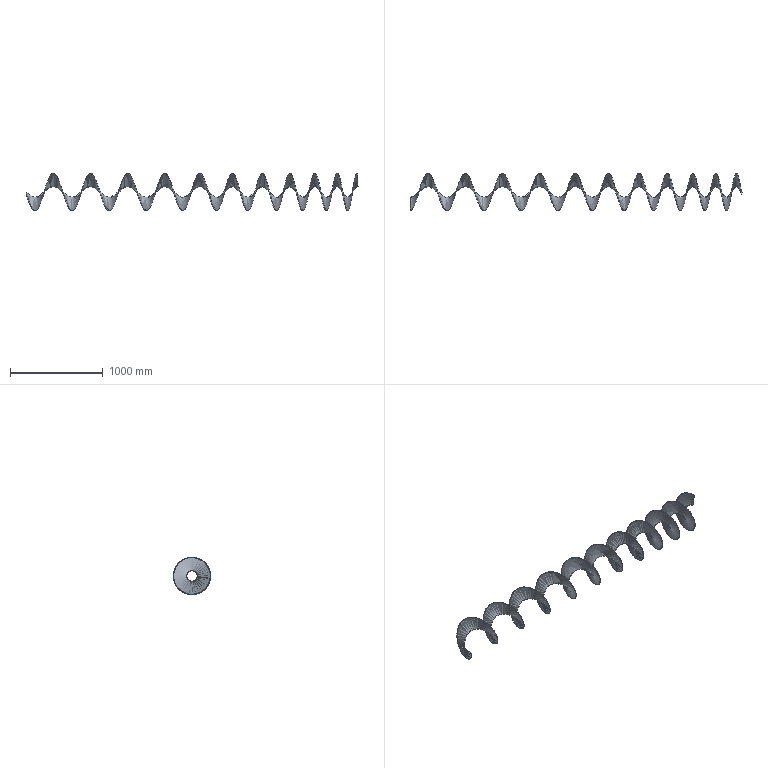Part | STEP file | Input 122 | 1 solid | 7 faces | box 3576 x 400.387 x 400.36 mm | volume 9588651 mm3 | spline 5 | plane 2